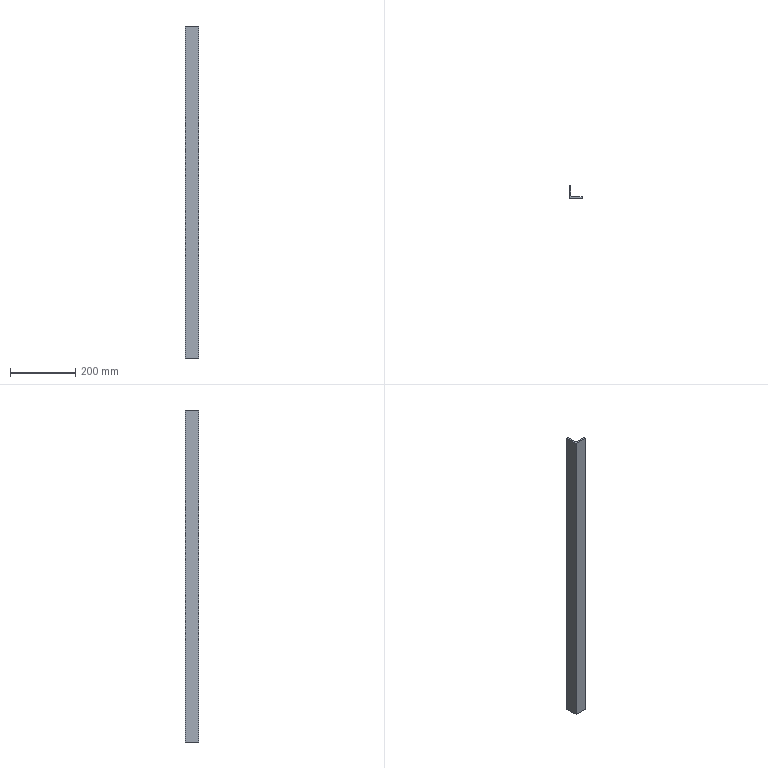Part | SolidWorks | features Extrusion 1 | 1 solid | 11 faces | box 40 x 40 x 1020 mm | volume 314774 mm3 | plane 8 | cylinder 3 | commonest cylinder face diameters 2.667 x2 10 x1
STEP:
#1=CARTESIAN_POINT('',(9.,4.,0.));
#2=VERTEX_POINT('',#1);
#3=CARTESIAN_POINT('',(4.,9.,0.));
#4=VERTEX_POINT('',#3);
#5=CARTESIAN_POINT('',(9.,9.,0.));
#6=DIRECTION('',(0.,0.,-1.));
#7=DIRECTION('',(-1.,0.,0.));
#8=AXIS2_PLACEMENT_3D('',#5,#6,#7);
#9=CIRCLE('',#8,5.);
#10=EDGE_CURVE('',#2,#4,#9,.T.);
#11=ORIENTED_EDGE('',*,*,#10,.T.);
#12=CARTESIAN_POINT('',(4.,9.,1020.));
#13=VERTEX_POINT('',#12);
#14=CARTESIAN_POINT('',(4.,9.,1020.));
#15=DIRECTION('',(0.,0.,-1.));
#16=VECTOR('',#15,1000.);
#17=LINE('',#14,#16);
#18=EDGE_CURVE('',#13,#4,#17,.T.);
#19=ORIENTED_EDGE('',*,*,#18,.F.);
#20=CARTESIAN_POINT('',(9.,4.,1020.));
#21=VERTEX_POINT('',#20);
#22=CARTESIAN_POINT('',(9.,9.,1020.));
#23=DIRECTION('',(0.,0.,-1.));
#24=DIRECTION('',(-1.,0.,0.));
#25=AXIS2_PLACEMENT_3D('',#22,#23,#24);
#26=CIRCLE('',#25,5.);
#27=EDGE_CURVE('',#21,#13,#26,.T.);
#28=ORIENTED_EDGE('',*,*,#27,.F.);
#29=CARTESIAN_POINT('',(9.,4.,1020.));
#30=DIRECTION('',(0.,0.,-1.));
#31=VECTOR('',#30,1000.);
#32=LINE('',#29,#31);
#33=EDGE_CURVE('',#21,#2,#32,.T.);
#34=ORIENTED_EDGE('',*,*,#33,.T.);
#35=EDGE_LOOP('',(#11,#19,#28,#34));
#36=FACE_OUTER_BOUND('',#35,.T.);
#37=CARTESIAN_POINT('',(9.,9.,1020.));
#38=DIRECTION('',(0.,0.,-1.));
#39=DIRECTION('',(-1.,0.,0.));
#40=AXIS2_PLACEMENT_3D('',#37,#38,#39);
#41=CYLINDRICAL_SURFACE('',#40,5.);
#42=ADVANCED_FACE('',(#36),#41,.F.);
#43=CARTESIAN_POINT('',(4.,38.667,0.));
#44=VERTEX_POINT('',#43);
#45=CARTESIAN_POINT('',(4.,38.667,0.));
#46=DIRECTION('',(0.,-1.,0.));
#47=VECTOR('',#46,1000.);
#48=LINE('',#45,#47);
#49=EDGE_CURVE('',#44,#4,#48,.T.);
#50=ORIENTED_EDGE('',*,*,#49,.F.);
#51=CARTESIAN_POINT('',(4.,38.667,1020.));
#52=VERTEX_POINT('',#51);
#53=CARTESIAN_POINT('',(4.,38.667,1020.));
#54=DIRECTION('',(0.,0.,-1.));
#55=VECTOR('',#54,1000.);
#56=LINE('',#53,#55);
#57=EDGE_CURVE('',#52,#44,#56,.T.);
#58=ORIENTED_EDGE('',*,*,#57,.F.);
#59=CARTESIAN_POINT('',(4.,38.667,1020.));
#60=DIRECTION('',(0.,-1.,0.));
#61=VECTOR('',#60,1000.);
#62=LINE('',#59,#61);
#63=EDGE_CURVE('',#52,#13,#62,.T.);
#64=ORIENTED_EDGE('',*,*,#63,.T.);
#65=ORIENTED_EDGE('',*,*,#18,.T.);
#66=EDGE_LOOP('',(#50,#58,#64,#65));
#67=FACE_OUTER_BOUND('',#66,.T.);
#68=CARTESIAN_POINT('',(4.,38.667,1020.));
#69=DIRECTION('',(1.,0.,0.));
#70=DIRECTION('',(0.,1.,0.));
#71=AXIS2_PLACEMENT_3D('',#68,#69,#70);
#72=PLANE('',#71);
#73=ADVANCED_FACE('',(#67),#72,.T.);
#74=CARTESIAN_POINT('',(2.667,40.,0.));
#75=VERTEX_POINT('',#74);
#76=CARTESIAN_POINT('',(2.667,38.667,0.));
#77=DIRECTION('',(0.,0.,-1.));
#78=DIRECTION('',(-1.,0.,0.));
#79=AXIS2_PLACEMENT_3D('',#76,#77,#78);
#80=CIRCLE('',#79,1.333);
#81=EDGE_CURVE('',#75,#44,#80,.T.);
#82=ORIENTED_EDGE('',*,*,#81,.F.);
#83=CARTESIAN_POINT('',(2.667,40.,1020.));
#84=VERTEX_POINT('',#83);
#85=CARTESIAN_POINT('',(2.667,40.,1020.));
#86=DIRECTION('',(0.,0.,-1.));
#87=VECTOR('',#86,1000.);
#88=LINE('',#85,#87);
#89=EDGE_CURVE('',#84,#75,#88,.T.);
#90=ORIENTED_EDGE('',*,*,#89,.F.);
#91=CARTESIAN_POINT('',(2.667,38.667,1020.));
#92=DIRECTION('',(0.,0.,-1.));
#93=DIRECTION('',(-1.,0.,0.));
#94=AXIS2_PLACEMENT_3D('',#91,#92,#93);
#95=CIRCLE('',#94,1.333);
#96=EDGE_CURVE('',#84,#52,#95,.T.);
#97=ORIENTED_EDGE('',*,*,#96,.T.);
#98=ORIENTED_EDGE('',*,*,#57,.T.);
#99=EDGE_LOOP('',(#82,#90,#97,#98));
#100=FACE_OUTER_BOUND('',#99,.T.);
#101=CARTESIAN_POINT('',(2.667,38.667,1020.));
#102=DIRECTION('',(0.,0.,-1.));
#103=DIRECTION('',(-1.,0.,0.));
#104=AXIS2_PLACEMENT_3D('',#101,#102,#103);
#105=CYLINDRICAL_SURFACE('',#104,1.333);
#106=ADVANCED_FACE('',(#100),#105,.T.);
#107=CARTESIAN_POINT('',(0.,40.,0.));
#108=VERTEX_POINT('',#107);
#109=CARTESIAN_POINT('',(0.,40.,0.));
#110=DIRECTION('',(1.,0.,0.));
#111=VECTOR('',#110,1000.);
#112=LINE('',#109,#111);
#113=EDGE_CURVE('',#108,#75,#112,.T.);
#114=ORIENTED_EDGE('',*,*,#113,.F.);
#115=CARTESIAN_POINT('',(0.,40.,1020.));
#116=VERTEX_POINT('',#115);
#117=CARTESIAN_POINT('',(0.,40.,1020.));
#118=DIRECTION('',(0.,0.,-1.));
#119=VECTOR('',#118,1000.);
#120=LINE('',#117,#119);
#121=EDGE_CURVE('',#116,#108,#120,.T.);
#122=ORIENTED_EDGE('',*,*,#121,.F.);
#123=CARTESIAN_POINT('',(0.,40.,1020.));
#124=DIRECTION('',(1.,0.,0.));
#125=VECTOR('',#124,1000.);
#126=LINE('',#123,#125);
#127=EDGE_CURVE('',#116,#84,#126,.T.);
#128=ORIENTED_EDGE('',*,*,#127,.T.);
#129=ORIENTED_EDGE('',*,*,#89,.T.);
#130=EDGE_LOOP('',(#114,#122,#128,#129));
#131=FACE_OUTER_BOUND('',#130,.T.);
#132=CARTESIAN_POINT('',(0.,40.,1020.));
#133=DIRECTION('',(0.,1.,0.));
#134=DIRECTION('',(0.,0.,1.));
#135=AXIS2_PLACEMENT_3D('',#132,#133,#134);
#136=PLANE('',#135);
#137=ADVANCED_FACE('',(#131),#136,.T.);
#138=CARTESIAN_POINT('',(0.,0.,0.));
#139=VERTEX_POINT('',#138);
#140=CARTESIAN_POINT('',(0.,0.,0.));
#141=DIRECTION('',(0.,1.,0.));
#142=VECTOR('',#141,1000.);
#143=LINE('',#140,#142);
#144=EDGE_CURVE('',#139,#108,#143,.T.);
#145=ORIENTED_EDGE('',*,*,#144,.F.);
#146=CARTESIAN_POINT('',(0.,0.,1020.));
#147=VERTEX_POINT('',#146);
#148=CARTESIAN_POINT('',(0.,0.,1020.));
#149=DIRECTION('',(0.,0.,-1.));
#150=VECTOR('',#149,1000.);
#151=LINE('',#148,#150);
#152=EDGE_CURVE('',#147,#139,#151,.T.);
#153=ORIENTED_EDGE('',*,*,#152,.F.);
#154=CARTESIAN_POINT('',(0.,0.,1020.));
#155=DIRECTION('',(0.,1.,0.));
#156=VECTOR('',#155,1000.);
#157=LINE('',#154,#156);
#158=EDGE_CURVE('',#147,#116,#157,.T.);
#159=ORIENTED_EDGE('',*,*,#158,.T.);
#160=ORIENTED_EDGE('',*,*,#121,.T.);
#161=EDGE_LOOP('',(#145,#153,#159,#160));
#162=FACE_OUTER_BOUND('',#161,.T.);
#163=CARTESIAN_POINT('',(0.,0.,1020.));
#164=DIRECTION('',(-1.,0.,0.));
#165=DIRECTION('',(0.,0.,1.));
#166=AXIS2_PLACEMENT_3D('',#163,#164,#165);
#167=PLANE('',#166);
#168=ADVANCED_FACE('',(#162),#167,.T.);
#169=CARTESIAN_POINT('',(40.,0.,0.));
#170=VERTEX_POINT('',#169);
#171=CARTESIAN_POINT('',(40.,0.,0.));
#172=DIRECTION('',(-1.,0.,0.));
#173=VECTOR('',#172,1000.);
#174=LINE('',#171,#173);
#175=EDGE_CURVE('',#170,#139,#174,.T.);
#176=ORIENTED_EDGE('',*,*,#175,.F.);
#177=CARTESIAN_POINT('',(40.,0.,1020.));
#178=VERTEX_POINT('',#177);
#179=CARTESIAN_POINT('',(40.,0.,1020.));
#180=DIRECTION('',(0.,0.,-1.));
#181=VECTOR('',#180,1000.);
#182=LINE('',#179,#181);
#183=EDGE_CURVE('',#178,#170,#182,.T.);
#184=ORIENTED_EDGE('',*,*,#183,.F.);
#185=CARTESIAN_POINT('',(40.,0.,1020.));
#186=DIRECTION('',(-1.,0.,0.));
#187=VECTOR('',#186,1000.);
#188=LINE('',#185,#187);
#189=EDGE_CURVE('',#178,#147,#188,.T.);
#190=ORIENTED_EDGE('',*,*,#189,.T.);
#191=ORIENTED_EDGE('',*,*,#152,.T.);
#192=EDGE_LOOP('',(#176,#184,#190,#191));
#193=FACE_OUTER_BOUND('',#192,.T.);
#194=CARTESIAN_POINT('',(40.,0.,1020.));
#195=DIRECTION('',(0.,-1.,0.));
#196=DIRECTION('',(0.,0.,-1.));
#197=AXIS2_PLACEMENT_3D('',#194,#195,#196);
#198=PLANE('',#197);
#199=ADVANCED_FACE('',(#193),#198,.T.);
#200=CARTESIAN_POINT('',(40.,2.667,0.));
#201=VERTEX_POINT('',#200);
#202=CARTESIAN_POINT('',(40.,0.,0.));
#203=DIRECTION('',(0.,1.,0.));
#204=VECTOR('',#203,1000.);
#205=LINE('',#202,#204);
#206=EDGE_CURVE('',#170,#201,#205,.T.);
#207=ORIENTED_EDGE('',*,*,#206,.T.);
#208=CARTESIAN_POINT('',(40.,2.667,1020.));
#209=VERTEX_POINT('',#208);
#210=CARTESIAN_POINT('',(40.,2.667,1020.));
#211=DIRECTION('',(0.,0.,-1.));
#212=VECTOR('',#211,1000.);
#213=LINE('',#210,#212);
#214=EDGE_CURVE('',#209,#201,#213,.T.);
#215=ORIENTED_EDGE('',*,*,#214,.F.);
#216=CARTESIAN_POINT('',(40.,0.,1020.));
#217=DIRECTION('',(0.,1.,0.));
#218=VECTOR('',#217,1000.);
#219=LINE('',#216,#218);
#220=EDGE_CURVE('',#178,#209,#219,.T.);
#221=ORIENTED_EDGE('',*,*,#220,.F.);
#222=ORIENTED_EDGE('',*,*,#183,.T.);
#223=EDGE_LOOP('',(#207,#215,#221,#222));
#224=FACE_OUTER_BOUND('',#223,.T.);
#225=CARTESIAN_POINT('',(40.,0.,1020.));
#226=DIRECTION('',(-1.,0.,0.));
#227=DIRECTION('',(0.,-1.,0.));
#228=AXIS2_PLACEMENT_3D('',#225,#226,#227);
#229=PLANE('',#228);
#230=ADVANCED_FACE('',(#224),#229,.F.);
#231=CARTESIAN_POINT('',(38.667,4.,0.));
#232=VERTEX_POINT('',#231);
#233=CARTESIAN_POINT('',(38.667,2.667,0.));
#234=DIRECTION('',(0.,0.,1.));
#235=DIRECTION('',(1.,0.,0.));
#236=AXIS2_PLACEMENT_3D('',#233,#234,#235);
#237=CIRCLE('',#236,1.333);
#238=EDGE_CURVE('',#201,#232,#237,.T.);
#239=ORIENTED_EDGE('',*,*,#238,.T.);
#240=CARTESIAN_POINT('',(38.667,4.,1020.));
#241=VERTEX_POINT('',#240);
#242=CARTESIAN_POINT('',(38.667,4.,1020.));
#243=DIRECTION('',(0.,0.,-1.));
#244=VECTOR('',#243,1000.);
#245=LINE('',#242,#244);
#246=EDGE_CURVE('',#241,#232,#245,.T.);
#247=ORIENTED_EDGE('',*,*,#246,.F.);
#248=CARTESIAN_POINT('',(38.667,2.667,1020.));
#249=DIRECTION('',(0.,0.,1.));
#250=DIRECTION('',(1.,0.,0.));
#251=AXIS2_PLACEMENT_3D('',#248,#249,#250);
#252=CIRCLE('',#251,1.333);
#253=EDGE_CURVE('',#209,#241,#252,.T.);
#254=ORIENTED_EDGE('',*,*,#253,.F.);
#255=ORIENTED_EDGE('',*,*,#214,.T.);
#256=EDGE_LOOP('',(#239,#247,#254,#255));
#257=FACE_OUTER_BOUND('',#256,.T.);
#258=CARTESIAN_POINT('',(38.667,2.667,1020.));
#259=DIRECTION('',(0.,0.,-1.));
#260=DIRECTION('',(-1.,0.,0.));
#261=AXIS2_PLACEMENT_3D('',#258,#259,#260);
#262=CYLINDRICAL_SURFACE('',#261,1.333);
#263=ADVANCED_FACE('',(#257),#262,.T.);
#264=CARTESIAN_POINT('',(9.,4.,0.));
#265=DIRECTION('',(1.,0.,0.));
#266=VECTOR('',#265,1000.);
#267=LINE('',#264,#266);
#268=EDGE_CURVE('',#2,#232,#267,.T.);
#269=ORIENTED_EDGE('',*,*,#268,.F.);
#270=ORIENTED_EDGE('',*,*,#33,.F.);
#271=CARTESIAN_POINT('',(9.,4.,1020.));
#272=DIRECTION('',(1.,0.,0.));
#273=VECTOR('',#272,1000.);
#274=LINE('',#271,#273);
#275=EDGE_CURVE('',#21,#241,#274,.T.);
#276=ORIENTED_EDGE('',*,*,#275,.T.);
#277=ORIENTED_EDGE('',*,*,#246,.T.);
#278=EDGE_LOOP('',(#269,#270,#276,#277));
#279=FACE_OUTER_BOUND('',#278,.T.);
#280=CARTESIAN_POINT('',(9.,4.,1020.));
#281=DIRECTION('',(0.,1.,0.));
#282=DIRECTION('',(-1.,0.,0.));
#283=AXIS2_PLACEMENT_3D('',#280,#281,#282);
#284=PLANE('',#283);
#285=ADVANCED_FACE('',(#279),#284,.T.);
#286=ORIENTED_EDGE('',*,*,#27,.T.);
#287=ORIENTED_EDGE('',*,*,#63,.F.);
#288=ORIENTED_EDGE('',*,*,#96,.F.);
#289=ORIENTED_EDGE('',*,*,#127,.F.);
#290=ORIENTED_EDGE('',*,*,#158,.F.);
#291=ORIENTED_EDGE('',*,*,#189,.F.);
#292=ORIENTED_EDGE('',*,*,#220,.T.);
#293=ORIENTED_EDGE('',*,*,#253,.T.);
#294=ORIENTED_EDGE('',*,*,#275,.F.);
#295=EDGE_LOOP('',(#286,#287,#288,#289,#290,#291,#292,#293,#294));
#296=FACE_OUTER_BOUND('',#295,.T.);
#297=CARTESIAN_POINT('',(9.,9.,1020.));
#298=DIRECTION('',(0.,0.,-1.));
#299=DIRECTION('',(-1.,0.,0.));
#300=AXIS2_PLACEMENT_3D('',#297,#298,#299);
#301=PLANE('',#300);
#302=ADVANCED_FACE('',(#296),#301,.F.);
#303=ORIENTED_EDGE('',*,*,#10,.F.);
#304=ORIENTED_EDGE('',*,*,#268,.T.);
#305=ORIENTED_EDGE('',*,*,#238,.F.);
#306=ORIENTED_EDGE('',*,*,#206,.F.);
#307=ORIENTED_EDGE('',*,*,#175,.T.);
#308=ORIENTED_EDGE('',*,*,#144,.T.);
#309=ORIENTED_EDGE('',*,*,#113,.T.);
#310=ORIENTED_EDGE('',*,*,#81,.T.);
#311=ORIENTED_EDGE('',*,*,#49,.T.);
#312=EDGE_LOOP('',(#303,#304,#305,#306,#307,#308,#309,#310,#311));
#313=FACE_OUTER_BOUND('',#312,.T.);
#314=CARTESIAN_POINT('',(9.,9.,0.));
#315=DIRECTION('',(0.,0.,-1.));
#316=DIRECTION('',(-1.,0.,0.));
#317=AXIS2_PLACEMENT_3D('',#314,#315,#316);
#318=PLANE('',#317);
#319=ADVANCED_FACE('',(#313),#318,.T.);
#320=CLOSED_SHELL('',(#42,#73,#106,#137,#168,#199,#230,#263,#285,#302,#319));
#321=MANIFOLD_SOLID_BREP('',#320);
#322=CARTESIAN_POINT('',(0.,0.,0.));
#323=DIRECTION('',(0.,0.,1.));
#324=DIRECTION('',(1.,0.,0.));
#325=AXIS2_PLACEMENT_3D('',#322,#323,#324);
#326=(LENGTH_UNIT()NAMED_UNIT(*)SI_UNIT(.MILLI.,.METRE.));
#327=UNCERTAINTY_MEASURE_WITH_UNIT(LENGTH_MEASURE(0.00001),#326,'','');
#328=(NAMED_UNIT(*)PLANE_ANGLE_UNIT()SI_UNIT($,.RADIAN.));
#329=(NAMED_UNIT(*)SI_UNIT($,.STERADIAN.)SOLID_ANGLE_UNIT());
#330=(GEOMETRIC_REPRESENTATION_CONTEXT(3)GLOBAL_UNCERTAINTY_ASSIGNED_CONTEXT((#327))GLOBAL_UNIT_ASSIGNED_CONTEXT((#326,#328,#329))REPRESENTATION_CONTEXT('',''));
#331=ADVANCED_BREP_SHAPE_REPRESENTATION('',(#321,#325),#330);